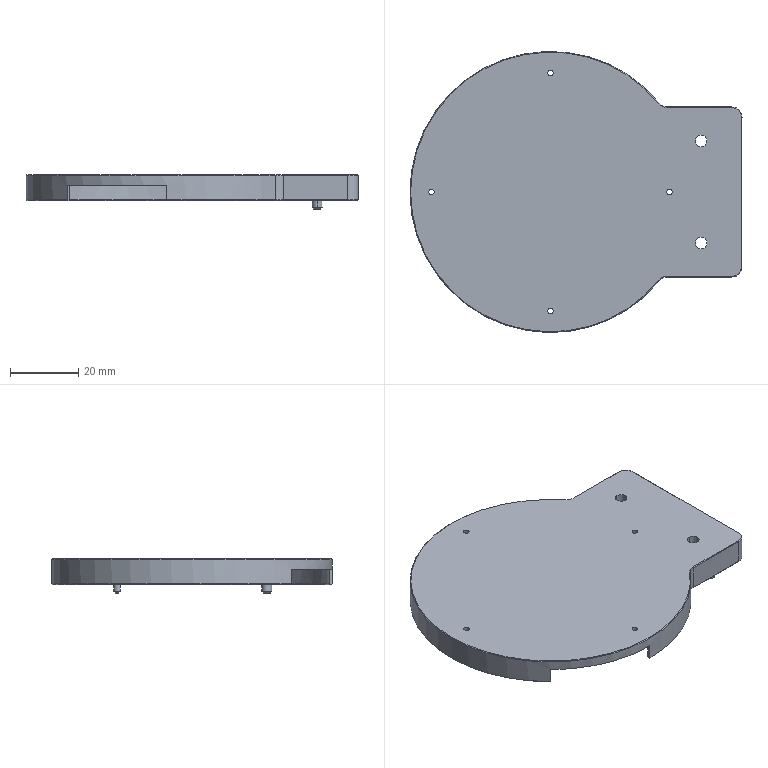NC program | NX | posted with a generic post | part box 97.6 x 82.6 x 10 mm
Lines 1 to 920 of 4898:
N10 G17 G21 G94 G90
(CAVITY_MILL , TOOL : D10)
N12 T15 M6
N14 G54
N16 G17 G0 G90 X-48.296 Y4.467 S9500 M3
N18 G43 Z30. H15
N20 Z0.7
N22 G94 G1 Z-0.8 F1000.
N24 X-42.296 Y7.931
N26 G3 X-41.796 Y8.797 R1.
N28 G1 X-1.296
N30 Y4.892 F2500.
N32 G2 X-0.532 Y4.504 R46.55
N34 X1.296 Y5.45 R47.05
N36 G1 Y8.797
N38 X-1.296
N40 Y13.297
N42 X-5.796
N44 Y2.003
N46 G2 X-0.481 Y-0.674 R42.05
N48 X5.796 Y2.544 R42.55
N50 G1 Y13.297
N52 X-1.296
N54 Y19.297
N56 X-8.082
N58 G3 X-11.796 Y15.583 R14.3
N60 G1 Y-0.583
N62 G3 X-9.863 Y-2.855 R14.3
N64 G2 X-0.413 Y-7.928 R36.05
N66 X10.632 Y-2.063 R36.55
N68 G3 X11.796 Y-0.583 R14.3
N70 G1 Y15.583
N72 G3 X8.082 Y19.297 R14.3
N74 G1 X-1.296
N76 Y25.297
N78 X-9.765
N80 G3 X-17.796 Y17.267 R20.3
N82 G1 Y-2.267
N84 G3 X-12.926 Y-8.153 R20.3
N86 G2 X-0.344 Y-15.967 R30.05
N88 X13.826 Y-7.364 R30.55
N90 G3 X17.796 Y-2.267 R20.3
N92 G1 Y17.267
N94 G3 X9.765 Y25.297 R20.3
N96 G1 X-1.296
N98 Y31.297
N100 X-11.198
N102 G3 X-23.796 Y18.7 R26.3
N104 G1 Y-3.7
N106 G3 X-16.623 Y-12.881 R26.3
N108 G2 X-15.848 Y-13.55 R18.
N110 X-0.276 Y-26.481 R24.05
N112 X16.681 Y-12.833 R24.55
N114 G3 X23.796 Y-3.7 R26.3
N116 G1 Y18.7
N118 G3 X11.198 Y31.297 R26.3
N120 G1 X-1.296
N122 Y37.297
N124 X-12.468
N126 G3 X-29.796 Y19.969 R32.3
N128 G1 Y-4.969
N130 G3 X-20.415 Y-17.53 R32.3
N132 G2 X-18.888 Y-19.02 R12.
N134 X-3.957 Y-37.297 R18.05
N136 G1 X3.457
N138 G2 X19.431 Y-18.429 R18.55
N140 X20.415 Y-17.53 R12.
N142 G3 X29.796 Y-4.969 R32.3
N144 G1 Y19.969
N146 G3 X12.468 Y37.297 R32.3
N148 G1 X-1.296
N150 Y43.297
N152 X-13.619
N154 G3 X-35.796 Y21.121 R38.3
N156 G1 Y-6.121
N158 G3 X-24.208 Y-22.18 R38.3
N160 G2 X-22.37 Y-24.756 R6.
N162 X-11.851 Y-43.297 R12.05
N164 G1 X11.263
N166 G2 X22.576 Y-24.263 R12.55
N168 X24.208 Y-22.18 R6.
N170 G3 X35.796 Y-6.121 R38.3
N172 G1 Y21.121
N174 G3 X13.619 Y43.297 R38.3
N176 G1 X-1.296
N178 Y49.297
N180 X-14.68
N182 G3 X-41.796 Y22.182 R44.3
N184 G1 Y-7.182
N186 G3 X-28. Y-26.829 R44.3
N188 G1 Y-32.73
N190 Y-36.024
N192 G2 X-24.748 Y-42.19 R-6.05
N194 X-28. Y-37.581 R6.051
N196 G1 Y-45.8
N198 G3 X-26.876 Y-49.297 R6.
N200 G1 X26.876
N202 G3 X28. Y-45.8 R6.
N204 G1 Y-41.705
N206 Y-39.427
N208 G2 X22.301 Y-30.257 R-6.55
N210 X28. Y-34.171 R6.551
N212 G1 Y-26.829
N214 G3 X41.796 Y-7.182 R44.3
N216 G1 Y22.182
N218 G3 X14.68 Y49.297 R44.3
N220 G1 X-1.296
N222 G2 X-2.162 Y49.797 R1.
N224 G1 X-5.626 Y55.797
N226 Z0.7
N228 G0 X-48.296 Y4.467 Z-0.1
N230 G1 Z-1.6 F1000.
N232 X-42.296 Y7.931
N234 G3 X-41.796 Y8.797 R1.
N236 G1 X-1.296
N238 Y4.893 F2500.
N240 G2 X-0.532 Y4.504 R46.55
N242 X1.296 Y5.45 R47.05
N244 G1 Y8.797
N246 X-1.296
N248 X-5.796
N250 Y2.003
N252 G2 X-0.481 Y-0.674 R42.05
N254 X5.796 Y2.544 R42.55
N256 G1 Y13.297
N258 X-5.796
N260 Y8.797
N262 X-11.796
N264 Y-0.583
N266 G3 X-9.863 Y-2.855 R14.3
N268 G2 X-0.413 Y-7.928 R36.05
N270 X10.632 Y-2.063 R36.55
N272 G3 X11.796 Y-0.583 R14.3
N274 G1 Y15.583
N276 G3 X8.082 Y19.297 R14.3
N278 G1 X-8.082
N280 G3 X-11.796 Y15.583 R14.3
N282 G1 Y8.797
N284 X-17.796
N286 Y-2.266
N288 G3 X-12.926 Y-8.153 R20.3
N290 G2 X-0.344 Y-15.967 R30.05
N292 X13.826 Y-7.364 R30.55
N294 G3 X17.796 Y-2.266 R20.3
N296 G1 Y17.266
N298 G3 X9.765 Y25.297 R20.3
N300 G1 X-9.765
N302 G3 X-17.796 Y17.266 R20.3
N304 G1 Y8.797
N306 X-23.796
N308 Y-3.699
N310 G3 X-16.623 Y-12.881 R26.3
N312 G2 X-15.848 Y-13.55 R18.
N314 X-0.276 Y-26.481 R24.05
N316 X16.681 Y-12.833 R24.55
N318 G3 X23.796 Y-3.699 R26.3
N320 G1 Y18.699
N322 G3 X11.198 Y31.297 R26.3
N324 G1 X-11.198
N326 G3 X-23.796 Y18.699 R26.3
N328 G1 Y8.797
N330 X-29.796
N332 Y-4.968
N334 G3 X-20.415 Y-17.53 R32.3
N336 G2 X-18.888 Y-19.02 R12.
N338 X-3.957 Y-37.297 R18.05
N340 G1 X3.457
N342 G2 X19.431 Y-18.429 R18.55
N344 X20.415 Y-17.53 R12.
N346 G3 X29.796 Y-4.968 R32.3
N348 G1 Y19.968
N350 G3 X12.467 Y37.297 R32.3
N352 G1 X-12.467
N354 G3 X-29.796 Y19.968 R32.3
N356 G1 Y8.797
N358 X-35.796
N360 Y-6.12
N362 G3 X-24.208 Y-22.18 R38.3
N364 G2 X-22.37 Y-24.756 R6.
N366 X-11.852 Y-43.297 R12.05
N368 G1 X11.263
N370 G2 X22.576 Y-24.263 R12.55
N372 X24.208 Y-22.18 R6.
N374 G3 X35.796 Y-6.12 R38.3
N376 G1 Y21.12
N378 G3 X13.618 Y43.297 R38.3
N380 G1 X-13.618
N382 G3 X-35.796 Y21.12 R38.3
N384 G1 Y8.797
N386 X-41.796
N388 Y-7.181
N390 G3 X-28. Y-26.829 R44.3
N392 G1 Y-32.73
N394 Y-36.024
N396 G2 X-24.748 Y-42.19 R-6.05
N398 X-28. Y-37.581 R6.051
N400 G1 Y-45.8
N402 G3 X-26.875 Y-49.297 R6.
N404 G1 X26.875
N406 G3 X28. Y-45.8 R6.
N408 G1 Y-41.705
N410 Y-39.427
N412 G2 X22.301 Y-30.257 R-6.55
N414 X28. Y-34.171 R6.551
N416 G1 Y-26.829
N418 G3 X41.796 Y-7.181 R44.3
N420 G1 Y22.181
N422 G3 X14.68 Y49.297 R44.3
N424 G1 X-14.68
N426 G3 X-41.796 Y22.181 R44.3
N428 G1 Y8.797
N430 G2 X-42.296 Y7.931 R1.
N432 G1 X-48.296 Y4.467
N434 Z-0.1
N436 G0 X-48.297 Z-0.9
N438 G1 Z-2.4 F1000.
N440 X-42.297 Y7.931
N442 G3 X-41.797 Y8.797 R1.
N444 G1 X-1.297
N446 Y4.893 F2500.
N448 G2 X-0.532 Y4.504 R46.55
N450 X1.297 Y5.45 R47.05
N452 G1 Y8.797
N454 X-1.297
N456 X-5.797
N458 Y2.003
N460 G2 X-0.481 Y-0.674 R42.05
N462 X5.797 Y2.544 R42.55
N464 G1 Y13.297
N466 X-5.797
N468 Y8.797
N470 X-11.797
N472 Y-0.582
N474 G3 X-9.863 Y-2.855 R14.3
N476 G2 X-0.413 Y-7.928 R36.05
N478 X10.632 Y-2.063 R36.55
N480 G3 X11.797 Y-0.582 R14.3
N482 G1 Y15.582
N484 G3 X8.082 Y19.297 R14.3
N486 G1 X-8.082
N488 G3 X-11.797 Y15.582 R14.3
N490 G1 Y8.797
N492 X-17.797
N494 Y-2.265
N496 G3 X-12.926 Y-8.153 R20.3
N498 G2 X-0.344 Y-15.967 R30.05
N500 X13.826 Y-7.364 R30.55
N502 G3 X17.797 Y-2.265 R20.3
N504 G1 Y17.265
N506 G3 X9.764 Y25.297 R20.3
N508 G1 X-9.764
N510 G3 X-17.797 Y17.265 R20.3
N512 G1 Y8.797
N514 X-23.797
N516 Y-3.698
N518 G3 X-16.623 Y-12.881 R26.3
N520 G2 X-15.848 Y-13.55 R18.
N522 X-0.276 Y-26.481 R24.05
N524 X16.681 Y-12.833 R24.55
N526 G3 X23.797 Y-3.698 R26.3
N528 G1 Y18.698
N530 G3 X11.197 Y31.297 R26.3
N532 G1 X-11.197
N534 G3 X-23.797 Y18.698 R26.3
N536 G1 Y8.797
N538 X-29.797
N540 Y-4.968
N542 G3 X-20.415 Y-17.53 R32.3
N544 G2 X-18.888 Y-19.02 R12.
N546 X-3.957 Y-37.297 R18.05
N548 G1 X3.457
N550 G2 X19.431 Y-18.429 R18.55
N552 X20.415 Y-17.53 R12.
N554 G3 X29.797 Y-4.968 R32.3
N556 G1 Y19.968
N558 G3 X12.466 Y37.297 R32.3
N560 G1 X-12.466
N562 G3 X-29.797 Y19.968 R32.3
N564 G1 Y8.797
N566 X-35.797
N568 Y-6.119
N570 G3 X-24.208 Y-22.18 R38.3
N572 G2 X-22.37 Y-24.756 R6.
N574 X-11.852 Y-43.297 R12.05
N576 G1 X11.263
N578 G2 X22.576 Y-24.263 R12.55
N580 X24.208 Y-22.18 R6.
N582 G3 X35.797 Y-6.119 R38.3
N584 G1 Y21.119
N586 G3 X13.618 Y43.297 R38.3
N588 G1 X-13.618
N590 G3 X-35.797 Y21.119 R38.3
N592 G1 Y8.797
N594 X-41.797
N596 Y-7.18
N598 G3 X-28. Y-26.829 R44.3
N600 G1 Y-32.73
N602 Y-36.024
N604 G2 X-24.748 Y-42.19 R-6.05
N606 X-28. Y-37.581 R6.051
N608 G1 Y-40.87
N610 Y-45.8
N612 G3 X-26.875 Y-49.297 R6.
N614 G1 X26.875
N616 G3 X28. Y-45.8 R6.
N618 G1 Y-39.427
N620 G2 X26.945 Y-32.505 R-6.55
N622 X28. Y-34.171 R6.551
N624 G1 Y-31.895
N626 Y-26.829
N628 G3 X41.797 Y-7.18 R44.3
N630 G1 Y22.18
N632 G3 X14.679 Y49.297 R44.3
N634 G1 X-14.679
N636 G3 X-41.797 Y22.18 R44.3
N638 G1 Y8.797
N640 G2 X-42.297 Y7.931 R1.
N642 G1 X-48.297 Y4.467
N644 Z-0.9
N646 G0 X48.297 Y14.347 Z-1.8
N648 G1 Z-3.3 F1000.
N650 X40.973
N652 G3 X41.797 Y13.781 R1.
N654 G1 Y15.084
N656 G3 X41.309 Y15.1 R7.594
N658 G1 X40.3
N660 G3 X36.61 Y14.145 R7.596
N662 G1 X0.701 Y7.645
N664 Y7.79 F2500.
N666 X0.495 Y7.995
N668 G3 X0.7 Y7.5 R-0.7
N670 G1 X0.701 Y7.645
N672 X5.2 Y7.629
N674 G2 X5.268 Y9.682 R35.09
N676 X3.677 Y11.177 R35.1
N678 G3 X5.2 Y7.5 R-5.2
N680 G1 Y7.629
N682 X11.2 Y7.608
N684 G2 X11.599 Y12.305 R29.09
N686 X7.92 Y15.42 R29.1
N688 G3 X11.2 Y7.501 R-11.2
N690 G1 Y7.608
N692 X17.2 Y7.586
N694 G2 X18.509 Y15.167 R23.09
N696 X12.162 Y19.662 R23.1
N698 G3 X9.925 Y-6.548 R-17.2
N700 X17.2 Y7.586 R17.2
N702 G1 X23.2 Y7.565
N704 G2 X24.226 Y13.336 R17.09
N706 X27.572 Y18.921 R17.096
N708 X16.405 Y23.905 R17.1
N710 G3 X13.387 Y-11.448 R-23.2
N712 X23.2 Y7.565 R23.2
N714 G1 X29.2 Y7.543
N716 G2 X29.866 Y11.289 R11.09
N718 X35.797 Y17.647 R11.096
N720 G1 Y21.118
N722 G3 X33.49 Y26.083 R38.3
N724 G2 X20.648 Y28.148 R11.1
N726 G3 X16.849 Y-16.348 R-29.2
N728 X29.2 Y7.543 R29.2
N730 G1 X35.2 Y7.522
N732 G2 X35.506 Y9.241 R5.09
N734 X40.3 Y12.6 R5.096
N736 G1 X41.309
N738 G2 X44.094 Y11.772 R5.094
N740 G3 X43.928 Y13.229 R44.3
N742 X41.797 Y13.781 R6.294
N744 G1 Y22.179
N746 G3 X34.196 Y35.662 R44.3
N748 G2 X32.81 Y33.097 R5.1
N750 G1 X32.103 Y32.39
N752 G2 X24.89 Y32.39 R5.1
N754 G3 X20.311 Y-21.249 R-35.2
N756 X35.2 Y7.522 R35.2
N758 X34.703 Y8.39 R1.
N760 G1 Z-1.8
N762 G0 Z30.
N764 X48.298 Y14.347
N766 Z-2.7
N768 G1 Z-4.2 F1000.
N770 X40.973
N772 G3 X41.798 Y13.781 R1.
N774 G1 Y15.084
N776 G3 X41.312 Y15.1 R7.592
N778 G1 X40.3
N780 G3 X36.608 Y14.145 R7.593
N782 G1 X0.701 Y7.645
N784 Y7.79 F2500.
N786 X0.495 Y7.995
N788 G3 X0.7 Y7.5 R-0.7
N790 G1 X0.701 Y7.645
N792 X5.2 Y7.629
N794 G2 X5.268 Y9.682 R35.081
N796 X3.677 Y11.177 R35.1
N798 G3 X5.2 Y7.501 R-5.2
N800 G1 Y7.629
N802 X11.2 Y7.608
N804 G2 X11.599 Y12.305 R29.081
N806 X7.92 Y15.42 R29.1
N808 G3 X11.2 Y7.502 R-11.2
N810 G1 Y7.608
N812 X17.2 Y7.587
N814 G2 X18.509 Y15.167 R23.081
N816 X12.162 Y19.662 R23.1
N818 G3 X10.663 Y-5.996 R-17.2
N820 X17.2 Y7.587 R17.2
N822 G1 X23.2 Y7.566
N824 G2 X24.225 Y13.334 R17.081
N826 X27.571 Y18.921 R17.093
N828 X16.405 Y23.905 R17.1
N830 G3 X14.383 Y-10.704 R-23.2
N832 X23.2 Y7.566 R23.2
N834 G1 X29.2 Y7.545
N836 G2 X29.865 Y11.288 R11.081
N838 X35.798 Y17.648 R11.093
N840 G1 Y21.117
N842 G3 X33.49 Y26.083 R38.3
N844 G2 X20.648 Y28.148 R11.1
N846 G3 X18.102 Y-15.412 R-29.2
N848 X29.2 Y7.545 R29.2
N850 G1 X35.2 Y7.524
N852 G2 X35.506 Y9.241 R5.081
N854 X40.3 Y12.6 R5.093
N856 G1 X41.312
N858 G2 X44.093 Y11.773 R5.092
N860 G3 X43.928 Y13.23 R44.3
N862 X41.798 Y13.781 R6.292
N864 G1 Y22.178
N866 G3 X34.196 Y35.662 R44.3
N868 G2 X32.81 Y33.097 R5.1
N870 G1 X32.103 Y32.39
N872 G2 X24.89 Y32.39 R5.1
N874 G3 X21.822 Y-20.12 R-35.2
N876 X35.2 Y7.524 R35.2
N878 X34.703 Y8.392 R1.
N880 G1 Z-2.7
N882 G0 Z30.
N884 X48.298 Y14.347
N886 Z-3.6
N888 G1 Z-5.1 F1000.
N890 X40.973
N892 G3 X41.798 Y13.781 R1.
N894 G1 Y15.085
N896 G3 X41.314 Y15.1 R7.589
N898 G1 X40.302
N900 G3 X36.603 Y14.144 R7.586
N902 G1 X0.701 Y7.645
N904 Y7.79 F2500.
N906 X0.495 Y7.995
N908 G3 X0.7 Y7.5 R-0.7
N910 G1 X0.701 Y7.645
N912 X5.2 Y7.63
N914 G2 X5.267 Y9.682 R35.072
N916 X3.677 Y11.177 R35.1
N918 G3 X5.2 Y7.501 R-5.2
N920 G1 Y7.63
N922 X11.2 Y7.609
N924 G2 X11.598 Y12.305 R29.072
N926 X7.92 Y15.42 R29.1
N928 G3 X11.2 Y7.502 R-11.2
N930 G1 Y7.609
N932 X17.2 Y7.588
N934 G2 X18.508 Y15.167 R23.072
N936 X12.162 Y19.662 R23.1
N938 G3 X-7.799 Y-7.83 R-17.2
N940 X17.2 Y7.588 R17.2
N942 G1 X23.2 Y7.567
N944 G2 X24.223 Y13.33 R17.072
N946 X27.569 Y18.922 R17.086
N948 X16.405 Y23.905 R17.1
N950 G3 X-10.519 Y-13.178 R-23.2
N952 X23.2 Y7.567 R23.2
N954 G1 X29.2 Y7.547
N956 G2 X29.864 Y11.286 R11.072
N958 X35.798 Y17.65 R11.086
N960 G1 Y21.116
N962 G3 X33.49 Y26.083 R38.3
N964 G2 X20.648 Y28.148 R11.1
N966 G3 X-13.24 Y-18.526 R-29.2
N968 X29.2 Y7.547 R29.2
N970 G1 X35.2 Y7.526
N972 G2 X35.505 Y9.241 R5.072
N974 X40.3 Y12.6 R5.086
N976 G1 X41.314
N978 G2 X44.093 Y11.774 R5.089
N980 G3 X43.928 Y13.231 R44.3
N982 X41.798 Y13.781 R6.289
N984 G1 Y22.177
N986 G3 X34.196 Y35.662 R44.3
N988 G2 X32.81 Y33.097 R5.1
N990 G1 X32.103 Y32.39
N992 G2 X24.89 Y32.39 R5.1
N994 G3 X-15.96 Y-23.874 R-35.2
N996 X35.2 Y7.526 R35.2
N998 X34.703 Y8.394 R1.
N1000 G1 Z-3.6
N1002 G0 Z30.
N1004 X48.298 Y14.346
N1006 Z-4.5
N1008 G1 Z-6. F1000.
N1010 X40.973
N1012 G3 X41.798 Y13.782 R1.
N1014 G1 Y15.085
N1016 G3 X41.318 Y15.1 R7.585
N1018 G1 X40.303
N1020 G3 X36.599 Y14.144 R7.581
N1022 G1 X0.7 Y7.645
N1024 X0.701 Y7.79 F2500.
N1026 X0.495 Y7.995
N1028 G3 X0.7 Y7.5 R-0.7
N1030 G1 Y7.645
N1032 X5.2 Y7.63
N1034 G2 X5.267 Y9.683 R35.063
N1036 X3.677 Y11.177 R35.1
N1038 G3 X5.2 Y7.501 R-5.2
N1040 G1 Y7.63
N1042 X11.2 Y7.61
N1044 G2 X11.598 Y12.305 R29.063
N1046 X7.92 Y15.42 R29.1
N1048 G3 X11.2 Y7.503 R-11.2
N1050 G1 Y7.61
N1052 X17.2 Y7.589
N1054 G2 X18.508 Y15.167 R23.063
N1056 X12.162 Y19.662 R23.1
N1058 G3 X-7.799 Y-7.83 R-17.2
N1060 X17.2 Y7.589 R17.2
N1062 G1 X23.2 Y7.569
N1064 G2 X24.222 Y13.327 R17.063
N1066 X27.568 Y18.922 R17.081
N1068 X16.405 Y23.905 R17.1
N1070 G3 X-10.519 Y-13.178 R-23.2
N1072 X23.2 Y7.569 R23.2
N1074 G1 X29.2 Y7.548
N1076 G2 X29.864 Y11.284 R11.063
N1078 X35.798 Y17.651 R11.081
N1080 G1 Y21.115
N1082 G3 X33.49 Y26.083 R38.3
N1084 G2 X20.648 Y28.148 R11.1
N1086 G3 X-13.24 Y-18.526 R-29.2
N1088 X29.2 Y7.548 R29.2
N1090 G1 X35.2 Y7.528
N1092 G2 X35.505 Y9.241 R5.063
N1094 X40.3 Y12.6 R5.081
N1096 G1 X41.318
N1098 G2 X44.093 Y11.776 R5.085
N1100 G3 X43.928 Y13.233 R44.3
N1102 X41.798 Y13.782 R6.285
N1104 G1 Y22.176
N1106 G3 X34.196 Y35.662 R44.3
N1108 G2 X32.81 Y33.097 R5.1
N1110 G1 X32.103 Y32.39
N1112 G2 X24.89 Y32.39 R5.1
N1114 G3 X-15.96 Y-23.874 R-35.2
N1116 X35.2 Y7.528 R35.2
N1118 X34.703 Y8.396 R1.
N1120 G1 Z-4.5
N1122 G0 Z30.
N1124 X48.299 Y14.346
N1126 Z-5.4
N1128 G1 Z-6.9 F1000.
N1130 X40.973
N1132 G3 X41.799 Y13.782 R1.
N1134 G1 Y15.085
N1136 G3 X41.32 Y15.1 R7.583
N1138 G1 X40.304
N1140 G3 X36.596 Y14.143 R7.576
N1142 G1 X0.7 Y7.645
N1144 X0.701 Y7.79 F2500.
N1146 X0.495 Y7.995
N1148 G3 X0.7 Y7.5 R-0.7
N1150 G1 Y7.645
N1152 X5.2 Y7.63
N1154 G2 X5.267 Y9.683 R35.054
N1156 X3.677 Y11.177 R35.1
N1158 G3 X5.2 Y7.502 R-5.2
N1160 G1 Y7.63
N1162 X11.2 Y7.61
N1164 G2 X11.598 Y12.306 R29.054
N1166 X7.92 Y15.42 R29.1
N1168 G3 X11.2 Y7.504 R-11.2
N1170 G1 Y7.61
N1172 X17.2 Y7.59
N1174 G2 X18.508 Y15.168 R23.054
N1176 X12.162 Y19.662 R23.1
N1178 G3 X-7.799 Y-7.83 R-17.2
N1180 X17.2 Y7.59 R17.2
N1182 G1 X23.2 Y7.57
N1184 G2 X24.221 Y13.324 R17.054
N1186 X27.566 Y18.922 R17.076
N1188 X16.405 Y23.905 R17.1
N1190 G3 X-10.519 Y-13.178 R-23.2
N1192 X23.2 Y7.57 R23.2
N1194 G1 X29.2 Y7.55
N1196 G2 X29.863 Y11.283 R11.054
N1198 X35.799 Y17.652 R11.076
N1200 G1 Y21.114
N1202 G3 X33.49 Y26.083 R38.3
N1204 G2 X20.648 Y28.148 R11.1
N1206 G3 X-13.24 Y-18.526 R-29.2
N1208 X29.2 Y7.55 R29.2
N1210 G1 X35.2 Y7.53
N1212 G2 X35.505 Y9.241 R5.054
N1214 X40.3 Y12.6 R5.076
N1216 G1 X41.32
N1218 G2 X44.093 Y11.777 R5.083
N1220 G3 X43.927 Y13.233 R44.3
N1222 X41.799 Y13.782 R6.283
N1224 G1 Y22.175
N1226 G3 X34.196 Y35.662 R44.3
N1228 G2 X32.81 Y33.097 R5.1
N1230 G1 X32.103 Y32.39
N1232 G2 X24.89 Y32.39 R5.1
N1234 G3 X-15.96 Y-23.874 R-35.2
N1236 X35.2 Y7.53 R35.2
N1238 X34.703 Y8.398 R1.
N1240 G1 Z-5.4
N1242 G0 X0.683 Y10.894
N1244 G1 X0. Y10.87 Z-5.436 F1000.
N1246 X-2.238 Y10.949 Z-5.553
N1248 X-3.606 Y11.106 Z-5.625
N1250 X-3.449 Y9.738 Z-5.698
N1252 X-3.37 Y7.5 Z-5.815
N1254 X-3.449 Y5.262 Z-5.932
N1256 X-3.606 Y3.894 Z-6.004
N1258 X-2.238 Y4.051 Z-6.077
N1260 X0. Y4.13 Z-6.194
N1262 X2.238 Y4.051 Z-6.311
N1264 X3.606 Y3.894 Z-6.384
N1266 X3.449 Y5.262 Z-6.456
N1268 X3.37 Y7.5 Z-6.573
N1270 X3.449 Y9.738 Z-6.691
N1272 X3.606 Y11.106 Z-6.763
N1274 X2.238 Y10.949 Z-6.835
N1276 X0. Y10.87 Z-6.952
N1278 X-2.238 Y10.949 Z-7.07
N1280 X-3.606 Y11.106 Z-7.142
N1282 X-3.449 Y9.738 Z-7.214
N1284 X-3.37 Y7.5 Z-7.331
N1286 X-3.449 Y5.262 Z-7.449
N1288 X-3.606 Y3.894 Z-7.521
N1290 X-2.238 Y4.051 Z-7.593
N1292 X0. Y4.13 Z-7.71
N1294 X2.238 Y4.051 Z-7.828
N1296 X3.606 Y3.894 Z-7.9
N1298 G2 X3.606 Y11.106 R31.6 F2500.
N1300 X-3.606 Y11.106 R31.6
N1302 X-3.606 Y3.894 R31.6
N1304 X3.606 Y3.894 R31.6
N1306 G1 X9.567 Y4.578
N1308 G2 X12.364 Y19.457 R25.6
N1310 G3 X11.957 Y19.864 R17.2
N1312 G2 X-11.957 Y19.864 R25.6
N1314 G3 X-12.364 Y19.457 R17.2
N1316 G2 X-12.364 Y-4.457 R25.6
N1318 G3 X-11.957 Y-4.864 R17.2
N1320 G2 X11.957 Y-4.864 R25.6
N1322 G3 X12.364 Y-4.457 R17.2
N1324 G2 X9.567 Y4.578 R25.6
N1326 G1 X15.528 Y5.263
N1328 G2 X19.701 Y19.752 R19.6
N1330 G3 X12.252 Y27.201 R23.2
N1332 G2 X-12.252 Y27.201 R19.6
N1334 G3 X-19.701 Y19.752 R23.2
N1336 G2 X-19.701 Y-4.752 R19.6
N1338 G3 X-12.252 Y-12.201 R23.2
N1340 G2 X12.252 Y-12.201 R19.6
N1342 G3 X19.701 Y-4.752 R23.2
N1344 G2 X15.528 Y5.263 R19.6
N1346 G1 X21.489 Y5.948
N1348 G2 X27.038 Y18.526 R13.6
N1350 G3 X11.026 Y34.538 R29.2
N1352 G2 X-11.026 Y34.538 R13.6
N1354 G3 X-27.038 Y18.526 R29.2
N1356 G2 X-27.038 Y-3.526 R13.6
N1358 G3 X-11.026 Y-19.538 R29.2
N1360 G2 X11.026 Y-19.538 R13.6
N1362 G3 X27.038 Y-3.526 R29.2
N1364 G2 X21.489 Y5.948 R13.6
N1366 G1 X27.45 Y6.633
N1368 G2 X34.375 Y15.074 R7.6
N1370 G3 X7.574 Y41.875 R35.2
N1372 G2 X-7.574 Y41.875 R7.6
N1374 G3 X-34.375 Y15.074 R35.2
N1376 G2 X-34.375 Y-0.074 R7.6
N1378 G3 X-7.574 Y-26.875 R35.2
N1380 G2 X7.574 Y-26.875 R7.6
N1382 G3 X34.375 Y-0.074 R35.2
N1384 G2 X27.45 Y6.633 R7.6
N1386 G3 X26.854 Y7.436 R1.
N1388 G1 Z-6.4
N1390 G0 X0.683 Y10.894
N1392 G1 X0. Y10.87 Z-6.436 F1000.
N1394 X-2.238 Y10.949 Z-6.553
N1396 X-3.606 Y11.106 Z-6.625
N1398 X-3.449 Y9.738 Z-6.698
N1400 X-3.37 Y7.5 Z-6.815
N1402 X-3.449 Y5.262 Z-6.932
N1404 X-3.606 Y3.894 Z-7.004
N1406 X-2.238 Y4.051 Z-7.077
N1408 X0. Y4.13 Z-7.194
N1410 X2.238 Y4.051 Z-7.311
N1412 X3.606 Y3.894 Z-7.384
N1414 X3.449 Y5.262 Z-7.456
N1416 X3.37 Y7.5 Z-7.573
N1418 X3.449 Y9.738 Z-7.691
N1420 X3.606 Y11.106 Z-7.763
N1422 X2.238 Y10.949 Z-7.835
N1424 X0. Y10.87 Z-7.952
N1426 X-2.238 Y10.949 Z-8.07
N1428 X-3.606 Y11.106 Z-8.142
N1430 X-3.449 Y9.738 Z-8.214
N1432 X-3.37 Y7.5 Z-8.331
N1434 X-3.449 Y5.262 Z-8.449
N1436 X-3.606 Y3.894 Z-8.521
N1438 X-2.238 Y4.051 Z-8.593
N1440 X0. Y4.13 Z-8.71
N1442 X2.238 Y4.051 Z-8.828
N1444 X3.606 Y3.894 Z-8.9
N1446 G2 X3.606 Y11.106 R31.6 F2500.
N1448 X-3.606 Y11.106 R31.6
N1450 X-3.606 Y3.894 R31.6
N1452 X3.606 Y3.894 R31.6
N1454 G1 X9.567 Y4.578
N1456 G2 X12.364 Y19.457 R25.6
N1458 G3 X11.957 Y19.864 R17.2
N1460 G2 X-11.957 Y19.864 R25.6
N1462 G3 X-12.364 Y19.457 R17.2
N1464 G2 X-12.364 Y-4.457 R25.6
N1466 G3 X-11.957 Y-4.864 R17.2
N1468 G2 X11.957 Y-4.864 R25.6
N1470 G3 X12.364 Y-4.457 R17.2
N1472 G2 X9.567 Y4.578 R25.6
N1474 G1 X15.528 Y5.263
N1476 G2 X19.701 Y19.752 R19.6
N1478 G3 X12.252 Y27.201 R23.2
N1480 G2 X-12.252 Y27.201 R19.6
N1482 G3 X-19.701 Y19.752 R23.2
N1484 G2 X-19.701 Y-4.752 R19.6
N1486 G3 X-12.252 Y-12.201 R23.2
N1488 G2 X12.252 Y-12.201 R19.6
N1490 G3 X19.701 Y-4.752 R23.2
N1492 G2 X15.528 Y5.263 R19.6
N1494 G1 X21.489 Y5.948
N1496 G2 X27.038 Y18.526 R13.6
N1498 G3 X11.026 Y34.538 R29.2
N1500 G2 X-11.026 Y34.538 R13.6
N1502 G3 X-27.038 Y18.526 R29.2
N1504 G2 X-27.038 Y-3.526 R13.6
N1506 G3 X-11.026 Y-19.538 R29.2
N1508 G2 X11.026 Y-19.538 R13.6
N1510 G3 X27.038 Y-3.526 R29.2
N1512 G2 X21.489 Y5.948 R13.6
N1514 G1 X27.45 Y6.633
N1516 G2 X34.375 Y15.074 R7.6
N1518 G3 X7.574 Y41.875 R35.2
N1520 G2 X-7.574 Y41.875 R7.6
N1522 G3 X-34.375 Y15.074 R35.2
N1524 G2 X-34.375 Y-0.074 R7.6
N1526 G3 X-7.574 Y-26.875 R35.2
N1528 G2 X7.574 Y-26.875 R7.6
N1530 G3 X34.375 Y-0.074 R35.2
N1532 G2 X27.45 Y6.633 R7.6
N1534 G3 X26.854 Y7.436 R1.
N1536 G1 Z-7.4
N1538 G0 Z30.
N1540 X4.788 Y-42.7
N1542 Z-0.9
N1544 G1 X4.9 Z-0.906 F1000.
N1546 Y-38.641 Z-1.119
N1548 X3.241 Y-38.817 Z-1.206
N1550 X0. Y-38.93 Z-1.376
N1552 X-3.241 Y-38.817 Z-1.546
N1554 X-4.9 Y-38.641 Z-1.633
N1556 Y-42.7 Z-1.846
N1558 X4.9 Z-2.36
N1560 Y-38.641 Z-2.572
N1562 X3.241 Y-38.817 Z-2.66
N1564 X0. Y-38.93 Z-2.83
N1566 X-3.241 Y-38.817 Z-3.
N1568 X-4.9 Y-38.641 Z-3.087
N1570 Y-42.7 Z-3.3
N1572 X4.9 F2500.
N1574 Y-38.641
N1576 G2 X-4.9 Y-38.641 R46.4
N1578 G1 Y-42.7
N1580 G3 X-4.034 Y-42.2 R1.
N1582 G1 Z-1.8
N1584 G0 X4.788 Y-42.7
N1586 G1 X4.9 Z-1.806 F1000.
N1588 Y-38.641 Z-2.019
N1590 X3.241 Y-38.817 Z-2.106
N1592 X0. Y-38.93 Z-2.276
N1594 X-3.241 Y-38.817 Z-2.446
N1596 X-4.9 Y-38.641 Z-2.533
N1598 Y-42.7 Z-2.746
N1600 X4.9 Z-3.26
N1602 Y-38.641 Z-3.472
N1604 X3.241 Y-38.817 Z-3.56
N1606 X0. Y-38.93 Z-3.73
N1608 X-3.241 Y-38.817 Z-3.9
N1610 X-4.9 Y-38.641 Z-3.987
N1612 Y-42.7 Z-4.2
N1614 X4.9 F2500.
N1616 Y-38.641
N1618 G2 X-4.9 Y-38.641 R46.4
N1620 G1 Y-42.7
N1622 G3 X-4.034 Y-42.2 R1.
N1624 G1 Z-2.7
N1626 G0 X4.788 Y-42.7
N1628 G1 X4.9 Z-2.706 F1000.
N1630 Y-38.641 Z-2.919
N1632 X3.241 Y-38.817 Z-3.006
N1634 X0. Y-38.93 Z-3.176
N1636 X-3.241 Y-38.817 Z-3.346
N1638 X-4.9 Y-38.641 Z-3.433
N1640 Y-42.7 Z-3.646
N1642 X4.9 Z-4.16
N1644 Y-38.641 Z-4.372
N1646 X3.241 Y-38.817 Z-4.46
N1648 X0. Y-38.93 Z-4.63
N1650 X-3.241 Y-38.817 Z-4.8
N1652 X-4.9 Y-38.641 Z-4.887
N1654 Y-42.7 Z-5.1
N1656 X4.9 F2500.
N1658 Y-38.641
N1660 G2 X-4.9 Y-38.641 R46.4
N1662 G1 Y-42.7
N1664 G3 X-4.034 Y-42.2 R1.
N1666 G1 Z-3.6
N1668 G0 X4.788 Y-42.7
N1670 G1 X4.9 Z-3.606 F1000.
N1672 Y-38.641 Z-3.819
N1674 X3.241 Y-38.817 Z-3.906
N1676 X0. Y-38.93 Z-4.076
N1678 X-3.241 Y-38.817 Z-4.246
N1680 X-4.9 Y-38.641 Z-4.333
N1682 Y-42.7 Z-4.546
N1684 X4.9 Z-5.06
N1686 Y-38.641 Z-5.272
N1688 X3.241 Y-38.817 Z-5.36
N1690 X0. Y-38.93 Z-5.53
N1692 X-3.241 Y-38.817 Z-5.7
N1694 X-4.9 Y-38.641 Z-5.787
N1696 Y-42.7 Z-6.
N1698 X4.9 F2500.
N1700 Y-38.641
N1702 G2 X-4.9 Y-38.641 R46.4
N1704 G1 Y-42.7
N1706 G3 X-4.034 Y-42.2 R1.
N1708 G1 Z-4.5
N1710 G0 X4.788 Y-42.7
N1712 G1 X4.9 Z-4.506 F1000.
N1714 Y-38.641 Z-4.719
N1716 X3.241 Y-38.817 Z-4.806
N1718 X0. Y-38.93 Z-4.976
N1720 X-3.241 Y-38.817 Z-5.146
N1722 X-4.9 Y-38.641 Z-5.233
N1724 Y-42.7 Z-5.446
N1726 X4.9 Z-5.96
N1728 Y-38.641 Z-6.172
N1730 X3.241 Y-38.817 Z-6.26
N1732 X0. Y-38.93 Z-6.43
N1734 X-3.241 Y-38.817 Z-6.6
N1736 X-4.9 Y-38.641 Z-6.687
N1738 Y-42.7 Z-6.9
N1740 X4.9 F2500.
N1742 Y-38.641
N1744 G2 X-4.9 Y-38.641 R46.4
N1746 G1 Y-42.7
N1748 G3 X-4.034 Y-42.2 R1.
N1750 G1 Z-5.4
N1752 G0 X2.88 Y-42.7
N1754 G1 X4.9 Z-5.506 F1000.
N1756 Y-38.641 Z-5.719
N1758 X3.241 Y-38.817 Z-5.806
N1760 X0. Y-38.93 Z-5.976
N1762 X-3.241 Y-38.817 Z-6.146
N1764 X-4.9 Y-38.641 Z-6.233
N1766 Y-42.7 Z-6.446
N1768 X4.9 Z-6.96
N1770 Y-38.641 Z-7.172
N1772 X3.241 Y-38.817 Z-7.26
N1774 X0. Y-38.93 Z-7.43
N1776 X-3.241 Y-38.817 Z-7.6
N1778 X-4.9 Y-38.641 Z-7.687
N1780 Y-42.7 Z-7.9
N1782 X4.9 F2500.
N1784 Y-38.641
N1786 G2 X-4.9 Y-38.641 R46.4
N1788 G1 Y-42.7
N1790 G3 X-4.034 Y-42.2 R1.
N1792 G1 Z-6.4
N1794 G0 X2.88 Y-42.7
N1796 G1 X4.9 Z-6.506 F1000.
N1798 Y-38.641 Z-6.719
N1800 X3.241 Y-38.817 Z-6.806
N1802 X0. Y-38.93 Z-6.976
N1804 X-3.241 Y-38.817 Z-7.146
N1806 X-4.9 Y-38.641 Z-7.233
N1808 Y-42.7 Z-7.446
N1810 X4.9 Z-7.96
N1812 Y-38.641 Z-8.172
N1814 X3.241 Y-38.817 Z-8.26
N1816 X0. Y-38.93 Z-8.43
N1818 X-3.241 Y-38.817 Z-8.6
N1820 X-4.9 Y-38.641 Z-8.687
N1822 Y-42.7 Z-8.9
N1824 X4.9 F2500.
N1826 Y-38.641
N1828 G2 X-4.9 Y-38.641 R46.4
N1830 G1 Y-42.7
N1832 G3 X-4.034 Y-42.2 R1.
N1834 G1 Z-7.4
N1836 G0 Z30.
N1838 M5